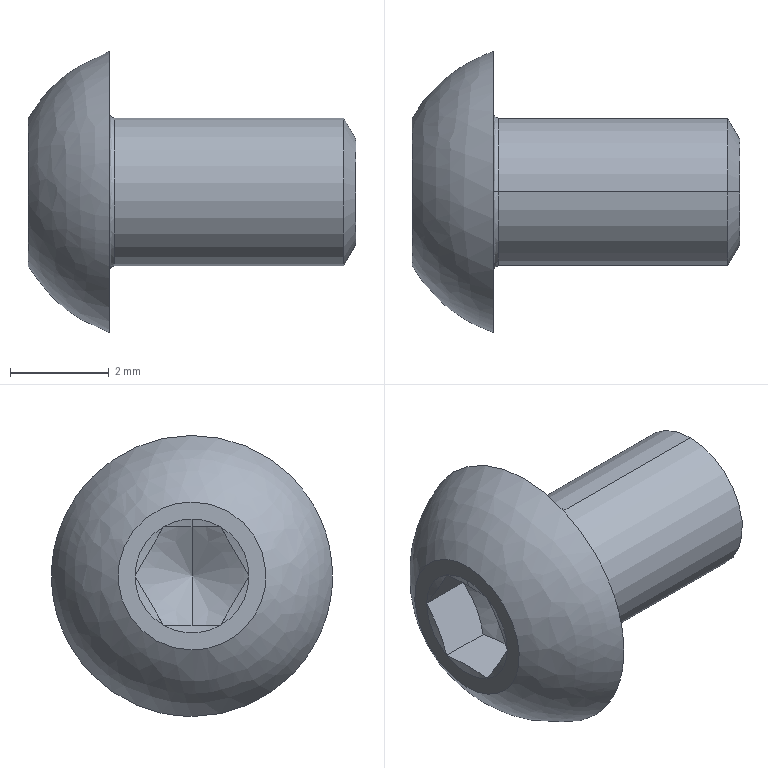Part | SolidWorks | features BaseBody 1 | 1 solid | 25 faces | box 6.65 x 5.7 x 5.7 mm | volume 59.694 mm3 | cone 11 | plane 9 | spline 3 | cylinder 2 | commonest cylinder face diameters 3 x2
STEP:
#1=CARTESIAN_POINT('',(-4.9,0.,-1.5));
#2=VERTEX_POINT('',#1);
#3=CARTESIAN_POINT('',(-4.9,0.,1.5));
#4=VERTEX_POINT('',#3);
#5=CARTESIAN_POINT('',(-4.9,0.,0.));
#6=DIRECTION('',(1.,0.,0.));
#7=DIRECTION('',(0.,0.,1.));
#8=AXIS2_PLACEMENT_3D('',#5,#6,#7);
#9=CIRCLE('',#8,1.5);
#10=EDGE_CURVE('',#2,#4,#9,.T.);
#11=ORIENTED_EDGE('',*,*,#10,.F.);
#12=CARTESIAN_POINT('',(-5.,0.,-1.6));
#13=VERTEX_POINT('',#12);
#14=CARTESIAN_POINT('',(-4.9,0.,-1.6));
#15=DIRECTION('',(0.,-1.,0.));
#16=DIRECTION('',(0.,0.,-1.));
#17=AXIS2_PLACEMENT_3D('',#14,#15,#16);
#18=CIRCLE('',#17,0.1);
#19=EDGE_CURVE('',#2,#13,#18,.T.);
#20=ORIENTED_EDGE('',*,*,#19,.T.);
#21=CARTESIAN_POINT('',(-5.,0.,1.6));
#22=VERTEX_POINT('',#21);
#23=CARTESIAN_POINT('',(-5.,0.,1.6));
#24=CARTESIAN_POINT('',(-5.,0.1018,1.6));
#25=CARTESIAN_POINT('',(-5.,0.2518,1.586));
#26=CARTESIAN_POINT('',(-5.,0.422,1.545));
#27=CARTESIAN_POINT('',(-5.,0.4939,1.522));
#28=CARTESIAN_POINT('',(-5.,0.5416,1.506));
#29=CARTESIAN_POINT('',(-5.,0.5632,1.498));
#30=CARTESIAN_POINT('',(-5.,0.7947,1.406));
#31=CARTESIAN_POINT('',(-5.,0.975,1.288));
#32=CARTESIAN_POINT('',(-5.,1.21,1.053));
#33=CARTESIAN_POINT('',(-5.,1.313,0.9266));
#34=CARTESIAN_POINT('',(-5.,1.408,0.7631));
#35=CARTESIAN_POINT('',(-5.,1.444,0.6896));
#36=CARTESIAN_POINT('',(-5.,1.467,0.6398));
#37=CARTESIAN_POINT('',(-5.,1.478,0.6126));
#38=CARTESIAN_POINT('',(-5.,1.563,0.3994));
#39=CARTESIAN_POINT('',(-5.,1.6,0.2038));
#40=CARTESIAN_POINT('',(-5.,1.6,-0.1019));
#41=CARTESIAN_POINT('',(-5.,1.586,-0.252));
#42=CARTESIAN_POINT('',(-5.,1.545,-0.4221));
#43=CARTESIAN_POINT('',(-5.,1.518,-0.5059));
#44=CARTESIAN_POINT('',(-5.,1.506,-0.5416));
#45=CARTESIAN_POINT('',(-5.,1.497,-0.5653));
#46=CARTESIAN_POINT('',(-5.,1.493,-0.5761));
#47=CARTESIAN_POINT('',(-5.,1.406,-0.7947));
#48=CARTESIAN_POINT('',(-5.,1.288,-0.975));
#49=CARTESIAN_POINT('',(-5.,1.053,-1.21));
#50=CARTESIAN_POINT('',(-5.,0.9266,-1.313));
#51=CARTESIAN_POINT('',(-5.,0.7631,-1.408));
#52=CARTESIAN_POINT('',(-5.,0.6896,-1.444));
#53=CARTESIAN_POINT('',(-5.,0.6398,-1.467));
#54=CARTESIAN_POINT('',(-5.,0.6126,-1.478));
#55=CARTESIAN_POINT('',(-5.,0.3994,-1.563));
#56=CARTESIAN_POINT('',(-5.,0.2038,-1.6));
#57=CARTESIAN_POINT('',(-5.,0.,-1.6));
#58=B_SPLINE_CURVE_WITH_KNOTS('',3,(#23,#24,#25,#26,#27,#28,#29,#30,#31,#32,#33,#34,#35,#36,#37,#38,#39,#40,#41,#42,#43,#44,#45,#46,#47,#48,#49,#50,#51,#52,#53,#54,#55,#56,#57),.UNSPECIFIED.,.F.,.F.,(4,1,1,2,2,2,1,1,2,2,2,1,1,1,2,2,2,1,1,2,2,4),(0.,0.03125,0.04688,0.05469,0.0625,0.125,0.1563,0.1719,0.1797,0.1875,0.25,0.2812,0.2969,0.3047,0.3086,0.3125,0.375,0.4062,0.4219,0.4297,0.4375,0.5),.UNSPECIFIED.);
#59=EDGE_CURVE('',#22,#13,#58,.T.);
#60=ORIENTED_EDGE('',*,*,#59,.F.);
#61=CARTESIAN_POINT('',(-4.9,0.,1.6));
#62=DIRECTION('',(0.,1.,0.));
#63=DIRECTION('',(0.,0.,1.));
#64=AXIS2_PLACEMENT_3D('',#61,#62,#63);
#65=CIRCLE('',#64,0.1);
#66=EDGE_CURVE('',#4,#22,#65,.T.);
#67=ORIENTED_EDGE('',*,*,#66,.F.);
#68=EDGE_LOOP('',(#11,#20,#60,#67));
#69=FACE_OUTER_BOUND('',#68,.T.);
#70=CARTESIAN_POINT('',(-4.9,0.,1.5));
#71=CARTESIAN_POINT('',(-4.9,3.,1.5));
#72=CARTESIAN_POINT('',(-4.9,3.,-1.5));
#73=CARTESIAN_POINT('',(-4.9,0.,-1.5));
#74=CARTESIAN_POINT('',(-4.959,0.,1.5));
#75=CARTESIAN_POINT('',(-4.959,3.,1.5));
#76=CARTESIAN_POINT('',(-4.959,3.,-1.5));
#77=CARTESIAN_POINT('',(-4.959,0.,-1.5));
#78=CARTESIAN_POINT('',(-5.,0.,1.541));
#79=CARTESIAN_POINT('',(-5.,3.083,1.541));
#80=CARTESIAN_POINT('',(-5.,3.083,-1.541));
#81=CARTESIAN_POINT('',(-5.,0.,-1.541));
#82=CARTESIAN_POINT('',(-5.,0.,1.6));
#83=CARTESIAN_POINT('',(-5.,3.2,1.6));
#84=CARTESIAN_POINT('',(-5.,3.2,-1.6));
#85=CARTESIAN_POINT('',(-5.,0.,-1.6));
#86=(BOUNDED_SURFACE()B_SPLINE_SURFACE(3,3,((#70,#71,#72,#73),(#74,#75,#76,#77),(#78,#79,#80,#81),(#82,#83,#84,#85)),.UNSPECIFIED.,.F.,.F.,.F.)B_SPLINE_SURFACE_WITH_KNOTS((4,4),(4,4),(0.,1.),(0.,1.),.UNSPECIFIED.)GEOMETRIC_REPRESENTATION_ITEM()RATIONAL_B_SPLINE_SURFACE(((1.,0.3333,0.3333,1.),(0.8047,0.2682,0.2682,0.8047),(0.8047,0.2682,0.2682,0.8047),(1.,0.3333,0.3333,1.)))REPRESENTATION_ITEM('')SURFACE());
#87=ADVANCED_FACE('',(#69),#86,.F.);
#88=CARTESIAN_POINT('',(-0.25,0.,1.5));
#89=VERTEX_POINT('',#88);
#90=CARTESIAN_POINT('',(-0.25,0.,-1.5));
#91=VERTEX_POINT('',#90);
#92=CARTESIAN_POINT('',(-0.25,0.,0.));
#93=DIRECTION('',(-1.,0.,0.));
#94=DIRECTION('',(0.,0.,1.));
#95=AXIS2_PLACEMENT_3D('',#92,#93,#94);
#96=CIRCLE('',#95,1.5);
#97=EDGE_CURVE('',#89,#91,#96,.T.);
#98=ORIENTED_EDGE('',*,*,#97,.T.);
#99=CARTESIAN_POINT('',(-6.65,0.,-1.5));
#100=DIRECTION('',(-1.,0.,0.));
#101=VECTOR('',#100,1000.);
#102=LINE('',#99,#101);
#103=EDGE_CURVE('',#91,#2,#102,.T.);
#104=ORIENTED_EDGE('',*,*,#103,.T.);
#105=ORIENTED_EDGE('',*,*,#10,.T.);
#106=CARTESIAN_POINT('',(-6.65,0.,1.5));
#107=DIRECTION('',(-1.,0.,0.));
#108=VECTOR('',#107,1000.);
#109=LINE('',#106,#108);
#110=EDGE_CURVE('',#89,#4,#109,.T.);
#111=ORIENTED_EDGE('',*,*,#110,.F.);
#112=EDGE_LOOP('',(#98,#104,#105,#111));
#113=FACE_OUTER_BOUND('',#112,.T.);
#114=CARTESIAN_POINT('',(-6.65,0.,0.));
#115=DIRECTION('',(-1.,0.,0.));
#116=DIRECTION('',(0.,0.,1.));
#117=AXIS2_PLACEMENT_3D('',#114,#115,#116);
#118=CYLINDRICAL_SURFACE('',#117,1.5);
#119=ADVANCED_FACE('',(#113),#118,.T.);
#120=CARTESIAN_POINT('',(0.,0.,1.067));
#121=VERTEX_POINT('',#120);
#122=CARTESIAN_POINT('',(0.,0.,-1.067));
#123=VERTEX_POINT('',#122);
#124=CARTESIAN_POINT('',(0.,0.,0.));
#125=DIRECTION('',(-1.,0.,0.));
#126=DIRECTION('',(0.,0.,1.));
#127=AXIS2_PLACEMENT_3D('',#124,#125,#126);
#128=CIRCLE('',#127,1.067);
#129=EDGE_CURVE('',#121,#123,#128,.T.);
#130=ORIENTED_EDGE('',*,*,#129,.T.);
#131=CARTESIAN_POINT('',(-0.25,0.,-1.5));
#132=DIRECTION('',(-0.5,0.,-0.866));
#133=VECTOR('',#132,1000.);
#134=LINE('',#131,#133);
#135=EDGE_CURVE('',#123,#91,#134,.T.);
#136=ORIENTED_EDGE('',*,*,#135,.T.);
#137=ORIENTED_EDGE('',*,*,#97,.F.);
#138=CARTESIAN_POINT('',(-0.25,0.,1.5));
#139=DIRECTION('',(-0.5,0.,0.866));
#140=VECTOR('',#139,1000.);
#141=LINE('',#138,#140);
#142=EDGE_CURVE('',#121,#89,#141,.T.);
#143=ORIENTED_EDGE('',*,*,#142,.F.);
#144=EDGE_LOOP('',(#130,#136,#137,#143));
#145=FACE_OUTER_BOUND('',#144,.T.);
#146=CARTESIAN_POINT('',(-0.25,0.,0.));
#147=DIRECTION('',(-1.,0.,0.));
#148=DIRECTION('',(0.,0.,1.));
#149=AXIS2_PLACEMENT_3D('',#146,#147,#148);
#150=CONICAL_SURFACE('',#149,1.5,1.047);
#151=ADVANCED_FACE('',(#145),#150,.T.);
#152=CARTESIAN_POINT('',(-6.61,0.,1.));
#153=VERTEX_POINT('',#152);
#154=CARTESIAN_POINT('',(-6.65,0.5774,1.));
#155=VERTEX_POINT('',#154);
#156=CARTESIAN_POINT('',(-6.61,0.,1.));
#157=CARTESIAN_POINT('',(-6.61,0.1925,1.));
#158=CARTESIAN_POINT('',(-6.625,0.3849,1.));
#159=CARTESIAN_POINT('',(-6.65,0.5774,1.));
#160=B_SPLINE_CURVE_WITH_KNOTS('',3,(#156,#157,#158,#159),.UNSPECIFIED.,.F.,.F.,(4,4),(0.0005774,0.001155),.UNSPECIFIED.);
#161=EDGE_CURVE('',#153,#155,#160,.T.);
#162=ORIENTED_EDGE('',*,*,#161,.F.);
#163=CARTESIAN_POINT('',(-6.65,0.,1.155));
#164=VERTEX_POINT('',#163);
#165=CARTESIAN_POINT('',(-6.65,0.,1.155));
#166=DIRECTION('',(-0.2515,0.,0.9679));
#167=VECTOR('',#166,1000.);
#168=LINE('',#165,#167);
#169=EDGE_CURVE('',#153,#164,#168,.T.);
#170=ORIENTED_EDGE('',*,*,#169,.T.);
#171=CARTESIAN_POINT('',(-6.65,0.,0.));
#172=DIRECTION('',(-1.,0.,0.));
#173=DIRECTION('',(0.,0.,1.));
#174=AXIS2_PLACEMENT_3D('',#171,#172,#173);
#175=CIRCLE('',#174,1.155);
#176=EDGE_CURVE('',#164,#155,#175,.T.);
#177=ORIENTED_EDGE('',*,*,#176,.T.);
#178=EDGE_LOOP('',(#162,#170,#177));
#179=FACE_OUTER_BOUND('',#178,.T.);
#180=CARTESIAN_POINT('',(-6.65,0.,0.));
#181=DIRECTION('',(-1.,0.,0.));
#182=DIRECTION('',(0.,0.,1.));
#183=AXIS2_PLACEMENT_3D('',#180,#181,#182);
#184=CONICAL_SURFACE('',#183,1.155,1.317);
#185=ADVANCED_FACE('',(#179),#184,.F.);
#186=CARTESIAN_POINT('',(-5.,0.,0.));
#187=VERTEX_POINT('',#186);
#188=CARTESIAN_POINT('',(-5.528,0.,1.));
#189=VERTEX_POINT('',#188);
#190=CARTESIAN_POINT('',(-5.614,0.,1.162));
#191=DIRECTION('',(-0.4671,0.,0.8842));
#192=VECTOR('',#191,1000.);
#193=LINE('',#190,#192);
#194=EDGE_CURVE('',#187,#189,#193,.T.);
#195=ORIENTED_EDGE('',*,*,#194,.F.);
#196=CARTESIAN_POINT('',(-5.528,0.,-1.));
#197=VERTEX_POINT('',#196);
#198=CARTESIAN_POINT('',(-5.614,0.,-1.162));
#199=DIRECTION('',(-0.4671,0.,-0.8842));
#200=VECTOR('',#199,1000.);
#201=LINE('',#198,#200);
#202=EDGE_CURVE('',#187,#197,#201,.T.);
#203=ORIENTED_EDGE('',*,*,#202,.T.);
#204=CARTESIAN_POINT('',(-5.61,-0.5774,-1.));
#205=VERTEX_POINT('',#204);
#206=CARTESIAN_POINT('',(-5.528,0.,-1.));
#207=CARTESIAN_POINT('',(-5.528,-0.1955,-1.));
#208=CARTESIAN_POINT('',(-5.56,-0.3883,-1.));
#209=CARTESIAN_POINT('',(-5.61,-0.5774,-1.));
#210=B_SPLINE_CURVE_WITH_KNOTS('',3,(#206,#207,#208,#209),.UNSPECIFIED.,.F.,.F.,(4,4),(0.0005831,0.001165),.UNSPECIFIED.);
#211=EDGE_CURVE('',#197,#205,#210,.T.);
#212=ORIENTED_EDGE('',*,*,#211,.T.);
#213=CARTESIAN_POINT('',(-5.61,-1.155,0.));
#214=VERTEX_POINT('',#213);
#215=CARTESIAN_POINT('',(-5.61,-0.5774,-1.));
#216=CARTESIAN_POINT('',(-5.56,-0.6719,-0.8362));
#217=CARTESIAN_POINT('',(-5.528,-0.7677,-0.6702));
#218=CARTESIAN_POINT('',(-5.528,-0.9635,-0.3311));
#219=CARTESIAN_POINT('',(-5.56,-1.06,-0.164));
#220=CARTESIAN_POINT('',(-5.61,-1.155,0.));
#221=B_SPLINE_CURVE_WITH_KNOTS('',3,(#215,#216,#217,#218,#219,#220),.UNSPECIFIED.,.F.,.F.,(4,2,4),(0.,0.0005823,0.001165),.UNSPECIFIED.);
#222=EDGE_CURVE('',#205,#214,#221,.T.);
#223=ORIENTED_EDGE('',*,*,#222,.T.);
#224=CARTESIAN_POINT('',(-5.61,-0.5774,1.));
#225=VERTEX_POINT('',#224);
#226=CARTESIAN_POINT('',(-5.61,-1.155,0.));
#227=CARTESIAN_POINT('',(-5.56,-1.06,0.1638));
#228=CARTESIAN_POINT('',(-5.528,-0.9643,0.3298));
#229=CARTESIAN_POINT('',(-5.528,-0.7685,0.6689));
#230=CARTESIAN_POINT('',(-5.56,-0.672,0.836));
#231=CARTESIAN_POINT('',(-5.61,-0.5774,1.));
#232=B_SPLINE_CURVE_WITH_KNOTS('',3,(#226,#227,#228,#229,#230,#231),.UNSPECIFIED.,.F.,.F.,(4,2,4),(0.,0.0005823,0.001165),.UNSPECIFIED.);
#233=EDGE_CURVE('',#214,#225,#232,.T.);
#234=ORIENTED_EDGE('',*,*,#233,.T.);
#235=CARTESIAN_POINT('',(-5.61,-0.5774,1.));
#236=CARTESIAN_POINT('',(-5.56,-0.3879,1.));
#237=CARTESIAN_POINT('',(-5.528,-0.1961,1.));
#238=CARTESIAN_POINT('',(-5.528,0.,1.));
#239=B_SPLINE_CURVE_WITH_KNOTS('',3,(#235,#236,#237,#238),.UNSPECIFIED.,.F.,.F.,(4,4),(0.,0.0005831),.UNSPECIFIED.);
#240=EDGE_CURVE('',#225,#189,#239,.T.);
#241=ORIENTED_EDGE('',*,*,#240,.T.);
#242=EDGE_LOOP('',(#195,#203,#212,#223,#234,#241));
#243=FACE_OUTER_BOUND('',#242,.T.);
#244=CARTESIAN_POINT('',(-5.614,0.,0.));
#245=DIRECTION('',(-1.,0.,0.));
#246=DIRECTION('',(0.,0.,1.));
#247=AXIS2_PLACEMENT_3D('',#244,#245,#246);
#248=CONICAL_SURFACE('',#247,1.162,1.085);
#249=ADVANCED_FACE('',(#243),#248,.F.);
#250=ORIENTED_EDGE('',*,*,#103,.F.);
#251=CARTESIAN_POINT('',(-0.25,0.,0.));
#252=DIRECTION('',(-1.,0.,0.));
#253=DIRECTION('',(0.,0.,1.));
#254=AXIS2_PLACEMENT_3D('',#251,#252,#253);
#255=CIRCLE('',#254,1.5);
#256=EDGE_CURVE('',#91,#89,#255,.T.);
#257=ORIENTED_EDGE('',*,*,#256,.T.);
#258=ORIENTED_EDGE('',*,*,#110,.T.);
#259=CARTESIAN_POINT('',(-4.9,0.,0.));
#260=DIRECTION('',(1.,0.,0.));
#261=DIRECTION('',(0.,0.,1.));
#262=AXIS2_PLACEMENT_3D('',#259,#260,#261);
#263=CIRCLE('',#262,1.5);
#264=EDGE_CURVE('',#4,#2,#263,.T.);
#265=ORIENTED_EDGE('',*,*,#264,.T.);
#266=EDGE_LOOP('',(#250,#257,#258,#265));
#267=FACE_OUTER_BOUND('',#266,.T.);
#268=CARTESIAN_POINT('',(-6.65,0.,0.));
#269=DIRECTION('',(-1.,0.,0.));
#270=DIRECTION('',(0.,0.,1.));
#271=AXIS2_PLACEMENT_3D('',#268,#269,#270);
#272=CYLINDRICAL_SURFACE('',#271,1.5);
#273=ADVANCED_FACE('',(#267),#272,.T.);
#274=ORIENTED_EDGE('',*,*,#135,.F.);
#275=CARTESIAN_POINT('',(0.,0.,0.));
#276=DIRECTION('',(-1.,0.,0.));
#277=DIRECTION('',(0.,0.,1.));
#278=AXIS2_PLACEMENT_3D('',#275,#276,#277);
#279=CIRCLE('',#278,1.067);
#280=EDGE_CURVE('',#123,#121,#279,.T.);
#281=ORIENTED_EDGE('',*,*,#280,.T.);
#282=ORIENTED_EDGE('',*,*,#142,.T.);
#283=ORIENTED_EDGE('',*,*,#256,.F.);
#284=EDGE_LOOP('',(#274,#281,#282,#283));
#285=FACE_OUTER_BOUND('',#284,.T.);
#286=CARTESIAN_POINT('',(-0.25,0.,0.));
#287=DIRECTION('',(-1.,0.,0.));
#288=DIRECTION('',(0.,0.,1.));
#289=AXIS2_PLACEMENT_3D('',#286,#287,#288);
#290=CONICAL_SURFACE('',#289,1.5,1.047);
#291=ADVANCED_FACE('',(#285),#290,.T.);
#292=ORIENTED_EDGE('',*,*,#19,.F.);
#293=ORIENTED_EDGE('',*,*,#264,.F.);
#294=ORIENTED_EDGE('',*,*,#66,.T.);
#295=CARTESIAN_POINT('',(-5.,0.,-1.6));
#296=CARTESIAN_POINT('',(-5.,-0.1019,-1.6));
#297=CARTESIAN_POINT('',(-5.,-0.252,-1.586));
#298=CARTESIAN_POINT('',(-5.,-0.4221,-1.545));
#299=CARTESIAN_POINT('',(-5.,-0.5059,-1.518));
#300=CARTESIAN_POINT('',(-5.,-0.5416,-1.506));
#301=CARTESIAN_POINT('',(-5.,-0.5653,-1.497));
#302=CARTESIAN_POINT('',(-5.,-0.5761,-1.493));
#303=CARTESIAN_POINT('',(-5.,-0.7947,-1.406));
#304=CARTESIAN_POINT('',(-5.,-0.975,-1.288));
#305=CARTESIAN_POINT('',(-5.,-1.21,-1.053));
#306=CARTESIAN_POINT('',(-5.,-1.313,-0.9266));
#307=CARTESIAN_POINT('',(-5.,-1.408,-0.7631));
#308=CARTESIAN_POINT('',(-5.,-1.444,-0.6896));
#309=CARTESIAN_POINT('',(-5.,-1.467,-0.6398));
#310=CARTESIAN_POINT('',(-5.,-1.478,-0.6126));
#311=CARTESIAN_POINT('',(-5.,-1.563,-0.3994));
#312=CARTESIAN_POINT('',(-5.,-1.6,-0.2038));
#313=CARTESIAN_POINT('',(-5.,-1.6,0.1019));
#314=CARTESIAN_POINT('',(-5.,-1.586,0.252));
#315=CARTESIAN_POINT('',(-5.,-1.545,0.4221));
#316=CARTESIAN_POINT('',(-5.,-1.518,0.5059));
#317=CARTESIAN_POINT('',(-5.,-1.506,0.5416));
#318=CARTESIAN_POINT('',(-5.,-1.497,0.5653));
#319=CARTESIAN_POINT('',(-5.,-1.493,0.5761));
#320=CARTESIAN_POINT('',(-5.,-1.406,0.7947));
#321=CARTESIAN_POINT('',(-5.,-1.288,0.975));
#322=CARTESIAN_POINT('',(-5.,-1.053,1.21));
#323=CARTESIAN_POINT('',(-5.,-0.9266,1.313));
#324=CARTESIAN_POINT('',(-5.,-0.7631,1.408));
#325=CARTESIAN_POINT('',(-5.,-0.6896,1.444));
#326=CARTESIAN_POINT('',(-5.,-0.6398,1.467));
#327=CARTESIAN_POINT('',(-5.,-0.6126,1.478));
#328=CARTESIAN_POINT('',(-5.,-0.3996,1.563));
#329=CARTESIAN_POINT('',(-5.,-0.2033,1.6));
#330=CARTESIAN_POINT('',(-5.,0.,1.6));
#331=B_SPLINE_CURVE_WITH_KNOTS('',3,(#295,#296,#297,#298,#299,#300,#301,#302,#303,#304,#305,#306,#307,#308,#309,#310,#311,#312,#313,#314,#315,#316,#317,#318,#319,#320,#321,#322,#323,#324,#325,#326,#327,#328,#329,#330),.UNSPECIFIED.,.F.,.F.,(4,1,1,1,2,2,2,1,1,2,2,2,1,1,1,2,2,2,1,1,2,2,4),(0.5,0.5312,0.5469,0.5547,0.5586,0.5625,0.625,0.6562,0.6719,0.6797,0.6875,0.75,0.7812,0.7969,0.8047,0.8086,0.8125,0.875,0.9062,0.9219,0.9297,0.9375,1.),.UNSPECIFIED.);
#332=EDGE_CURVE('',#13,#22,#331,.T.);
#333=ORIENTED_EDGE('',*,*,#332,.F.);
#334=EDGE_LOOP('',(#292,#293,#294,#333));
#335=FACE_OUTER_BOUND('',#334,.T.);
#336=CARTESIAN_POINT('',(-4.9,0.,-1.5));
#337=CARTESIAN_POINT('',(-4.9,-3.,-1.5));
#338=CARTESIAN_POINT('',(-4.9,-3.,1.5));
#339=CARTESIAN_POINT('',(-4.9,0.,1.5));
#340=CARTESIAN_POINT('',(-4.959,0.,-1.5));
#341=CARTESIAN_POINT('',(-4.959,-3.,-1.5));
#342=CARTESIAN_POINT('',(-4.959,-3.,1.5));
#343=CARTESIAN_POINT('',(-4.959,0.,1.5));
#344=CARTESIAN_POINT('',(-5.,0.,-1.541));
#345=CARTESIAN_POINT('',(-5.,-3.083,-1.541));
#346=CARTESIAN_POINT('',(-5.,-3.083,1.541));
#347=CARTESIAN_POINT('',(-5.,0.,1.541));
#348=CARTESIAN_POINT('',(-5.,0.,-1.6));
#349=CARTESIAN_POINT('',(-5.,-3.2,-1.6));
#350=CARTESIAN_POINT('',(-5.,-3.2,1.6));
#351=CARTESIAN_POINT('',(-5.,0.,1.6));
#352=(BOUNDED_SURFACE()B_SPLINE_SURFACE(3,3,((#336,#337,#338,#339),(#340,#341,#342,#343),(#344,#345,#346,#347),(#348,#349,#350,#351)),.UNSPECIFIED.,.F.,.F.,.F.)B_SPLINE_SURFACE_WITH_KNOTS((4,4),(4,4),(0.,1.),(0.,1.),.UNSPECIFIED.)GEOMETRIC_REPRESENTATION_ITEM()RATIONAL_B_SPLINE_SURFACE(((1.,0.3333,0.3333,1.),(0.8047,0.2682,0.2682,0.8047),(0.8047,0.2682,0.2682,0.8047),(1.,0.3333,0.3333,1.)))REPRESENTATION_ITEM('')SURFACE());
#353=ADVANCED_FACE('',(#335),#352,.F.);
#354=ORIENTED_EDGE('',*,*,#129,.F.);
#355=ORIENTED_EDGE('',*,*,#280,.F.);
#356=EDGE_LOOP('',(#354,#355));
#357=FACE_OUTER_BOUND('',#356,.T.);
#358=CARTESIAN_POINT('',(0.,1.5,0.));
#359=DIRECTION('',(-1.,0.,0.));
#360=DIRECTION('',(0.,0.,1.));
#361=AXIS2_PLACEMENT_3D('',#358,#359,#360);
#362=PLANE('',#361);
#363=ADVANCED_FACE('',(#357),#362,.F.);
#364=ORIENTED_EDGE('',*,*,#59,.T.);
#365=ORIENTED_EDGE('',*,*,#332,.T.);
#366=EDGE_LOOP('',(#364,#365));
#367=FACE_BOUND('',#366,.T.);
#368=CARTESIAN_POINT('',(-5.,0.,-2.85));
#369=VERTEX_POINT('',#368);
#370=CARTESIAN_POINT('',(-5.,0.001007,2.85));
#371=VERTEX_POINT('',#370);
#372=CARTESIAN_POINT('',(-5.,0.,-2.85));
#373=CARTESIAN_POINT('',(-5.,-0.3766,-2.85));
#374=CARTESIAN_POINT('',(-5.,-0.7506,-2.774));
#375=CARTESIAN_POINT('',(-5.,-1.265,-2.561));
#376=CARTESIAN_POINT('',(-5.,-1.431,-2.472));
#377=CARTESIAN_POINT('',(-5.,-1.742,-2.263));
#378=CARTESIAN_POINT('',(-5.,-1.885,-2.145));
#379=CARTESIAN_POINT('',(-5.,-2.148,-1.882));
#380=CARTESIAN_POINT('',(-5.,-2.269,-1.735));
#381=CARTESIAN_POINT('',(-5.,-2.475,-1.425));
#382=CARTESIAN_POINT('',(-5.,-2.562,-1.262));
#383=CARTESIAN_POINT('',(-5.,-2.705,-0.9158));
#384=CARTESIAN_POINT('',(-5.,-2.76,-0.7352));
#385=CARTESIAN_POINT('',(-5.,-2.832,-0.371));
#386=CARTESIAN_POINT('',(-5.,-2.85,-0.185));
#387=CARTESIAN_POINT('',(-5.,-2.85,0.1908));
#388=CARTESIAN_POINT('',(-5.,-2.831,0.3758));
#389=CARTESIAN_POINT('',(-5.,-2.758,0.7401));
#390=CARTESIAN_POINT('',(-5.,-2.703,0.9214));
#391=CARTESIAN_POINT('',(-5.,-2.56,1.266));
#392=CARTESIAN_POINT('',(-5.,-2.473,1.43));
#393=CARTESIAN_POINT('',(-5.,-2.265,1.74));
#394=CARTESIAN_POINT('',(-5.,-2.145,1.886));
#395=CARTESIAN_POINT('',(-5.,-1.882,2.148));
#396=CARTESIAN_POINT('',(-5.,-1.738,2.266));
#397=CARTESIAN_POINT('',(-5.,-1.426,2.475));
#398=CARTESIAN_POINT('',(-5.,-1.26,2.563));
#399=CARTESIAN_POINT('',(-5.,-0.9174,2.705));
#400=CARTESIAN_POINT('',(-5.,-0.7372,2.759));
#401=CARTESIAN_POINT('',(-5.,-0.3698,2.832));
#402=CARTESIAN_POINT('',(-5.,-0.185,2.85));
#403=CARTESIAN_POINT('',(-5.,0.001007,2.85));
#404=B_SPLINE_CURVE_WITH_KNOTS('',3,(#372,#373,#374,#375,#376,#377,#378,#379,#380,#381,#382,#383,#384,#385,#386,#387,#388,#389,#390,#391,#392,#393,#394,#395,#396,#397,#398,#399,#400,#401,#402,#403),.UNSPECIFIED.,.F.,.F.,(4,2,2,2,2,2,2,2,2,2,2,2,2,2,2,4),(0.,0.001123,0.001685,0.002247,0.002809,0.00337,0.003932,0.004494,0.005056,0.005617,0.006179,0.006741,0.007302,0.007864,0.008426,0.008988),.UNSPECIFIED.);
#405=EDGE_CURVE('',#369,#371,#404,.T.);
#406=ORIENTED_EDGE('',*,*,#405,.F.);
#407=CARTESIAN_POINT('',(-5.,0.001007,2.85));
#408=CARTESIAN_POINT('',(-5.,0.187,2.85));
#409=CARTESIAN_POINT('',(-5.,0.3759,2.831));
#410=CARTESIAN_POINT('',(-5.,0.741,2.758));
#411=CARTESIAN_POINT('',(-5.,0.9186,2.704));
#412=CARTESIAN_POINT('',(-5.,1.264,2.561));
#413=CARTESIAN_POINT('',(-5.,1.43,2.472));
#414=CARTESIAN_POINT('',(-5.,1.739,2.266));
#415=CARTESIAN_POINT('',(-5.,1.883,2.147));
#416=CARTESIAN_POINT('',(-5.,2.149,1.881));
#417=CARTESIAN_POINT('',(-5.,2.267,1.737));
#418=CARTESIAN_POINT('',(-5.,2.473,1.428));
#419=CARTESIAN_POINT('',(-5.,2.562,1.261));
#420=CARTESIAN_POINT('',(-5.,2.705,0.9163));
#421=CARTESIAN_POINT('',(-5.,2.759,0.7387));
#422=CARTESIAN_POINT('',(-5.,2.832,0.3731));
#423=CARTESIAN_POINT('',(-5.,2.85,0.1844));
#424=CARTESIAN_POINT('',(-5.,2.85,-0.1874));
#425=CARTESIAN_POINT('',(-5.,2.832,-0.3723));
#426=CARTESIAN_POINT('',(-5.,2.759,-0.7402));
#427=CARTESIAN_POINT('',(-5.,2.704,-0.9197));
#428=CARTESIAN_POINT('',(-5.,2.562,-1.263));
#429=CARTESIAN_POINT('',(-5.,2.473,-1.429));
#430=CARTESIAN_POINT('',(-5.,2.265,-1.74));
#431=CARTESIAN_POINT('',(-5.,2.147,-1.884));
#432=CARTESIAN_POINT('',(-5.,1.884,-2.147));
#433=CARTESIAN_POINT('',(-5.,1.737,-2.267));
#434=CARTESIAN_POINT('',(-5.,1.427,-2.474));
#435=CARTESIAN_POINT('',(-5.,1.264,-2.561));
#436=CARTESIAN_POINT('',(-5.,0.9187,-2.704));
#437=CARTESIAN_POINT('',(-5.,0.7377,-2.759));
#438=CARTESIAN_POINT('',(-5.,0.3734,-2.832));
#439=CARTESIAN_POINT('',(-5.,0.1883,-2.85));
#440=CARTESIAN_POINT('',(-5.,0.,-2.85));
#441=B_SPLINE_CURVE_WITH_KNOTS('',3,(#407,#408,#409,#410,#411,#412,#413,#414,#415,#416,#417,#418,#419,#420,#421,#422,#423,#424,#425,#426,#427,#428,#429,#430,#431,#432,#433,#434,#435,#436,#437,#438,#439,#440),.UNSPECIFIED.,.F.,.F.,(4,2,2,2,2,2,2,2,2,2,2,2,2,2,2,2,4),(0.008988,0.009549,0.01011,0.01067,0.01123,0.0118,0.01236,0.01292,0.01348,0.01404,0.0146,0.01517,0.01573,0.01629,0.01685,0.01741,0.01798),.UNSPECIFIED.);
#442=EDGE_CURVE('',#371,#369,#441,.T.);
#443=ORIENTED_EDGE('',*,*,#442,.F.);
#444=EDGE_LOOP('',(#406,#443));
#445=FACE_OUTER_BOUND('',#444,.T.);
#446=CARTESIAN_POINT('',(-5.,1.6,0.));
#447=DIRECTION('',(-1.,0.,0.));
#448=DIRECTION('',(0.,0.,1.));
#449=AXIS2_PLACEMENT_3D('',#446,#447,#448);
#450=PLANE('',#449);
#451=ADVANCED_FACE('',(#367,#445),#450,.F.);
#452=ORIENTED_EDGE('',*,*,#405,.T.);
#453=ORIENTED_EDGE('',*,*,#442,.T.);
#454=EDGE_LOOP('',(#452,#453));
#455=FACE_OUTER_BOUND('',#454,.T.);
#456=CARTESIAN_POINT('',(-6.65,0.,-1.5));
#457=VERTEX_POINT('',#456);
#458=CARTESIAN_POINT('',(-6.65,-0.0005302,1.5));
#459=VERTEX_POINT('',#458);
#460=CARTESIAN_POINT('',(-6.65,0.,-1.5));
#461=CARTESIAN_POINT('',(-6.65,0.1982,-1.5));
#462=CARTESIAN_POINT('',(-6.65,0.3951,-1.46));
#463=CARTESIAN_POINT('',(-6.65,0.756,-1.31));
#464=CARTESIAN_POINT('',(-6.65,0.9231,-1.198));
#465=CARTESIAN_POINT('',(-6.65,1.131,-0.9905));
#466=CARTESIAN_POINT('',(-6.65,1.194,-0.9132));
#467=CARTESIAN_POINT('',(-6.65,1.303,-0.7502));
#468=CARTESIAN_POINT('',(-6.65,1.349,-0.664));
#469=CARTESIAN_POINT('',(-6.65,1.461,-0.391));
#470=CARTESIAN_POINT('',(-6.65,1.5,-0.1963));
#471=CARTESIAN_POINT('',(-6.65,1.5,0.1004));
#472=CARTESIAN_POINT('',(-6.65,1.49,0.1978));
#473=CARTESIAN_POINT('',(-6.65,1.452,0.3895));
#474=CARTESIAN_POINT('',(-6.65,1.423,0.4849));
#475=CARTESIAN_POINT('',(-6.65,1.347,0.6663));
#476=CARTESIAN_POINT('',(-6.65,1.301,0.7524));
#477=CARTESIAN_POINT('',(-6.65,1.192,0.9155));
#478=CARTESIAN_POINT('',(-6.65,1.129,0.9926));
#479=CARTESIAN_POINT('',(-6.65,0.9212,1.2));
#480=CARTESIAN_POINT('',(-6.65,0.7537,1.312));
#481=CARTESIAN_POINT('',(-6.65,0.3926,1.461));
#482=CARTESIAN_POINT('',(-6.65,0.1952,1.5));
#483=CARTESIAN_POINT('',(-6.65,-0.0005302,1.5));
#484=B_SPLINE_CURVE_WITH_KNOTS('',3,(#460,#461,#462,#463,#464,#465,#466,#467,#468,#469,#470,#471,#472,#473,#474,#475,#476,#477,#478,#479,#480,#481,#482,#483),.UNSPECIFIED.,.F.,.F.,(4,2,2,2,2,2,2,2,2,2,2,4),(0.,0.0005913,0.001183,0.001478,0.001774,0.002365,0.002661,0.002956,0.003252,0.003548,0.004139,0.00473),.UNSPECIFIED.);
#485=EDGE_CURVE('',#457,#459,#484,.T.);
#486=ORIENTED_EDGE('',*,*,#485,.T.);
#487=CARTESIAN_POINT('',(-6.65,-0.0005302,1.5));
#488=CARTESIAN_POINT('',(-6.65,-0.09842,1.5));
#489=CARTESIAN_POINT('',(-6.65,-0.1978,1.49));
#490=CARTESIAN_POINT('',(-6.65,-0.39,1.452));
#491=CARTESIAN_POINT('',(-6.65,-0.4835,1.423));
#492=CARTESIAN_POINT('',(-6.65,-0.7562,1.31));
#493=CARTESIAN_POINT('',(-6.65,-0.9213,1.2));
#494=CARTESIAN_POINT('',(-6.65,-1.131,0.9901));
#495=CARTESIAN_POINT('',(-6.65,-1.193,0.9143));
#496=CARTESIAN_POINT('',(-6.65,-1.302,0.7517));
#497=CARTESIAN_POINT('',(-6.65,-1.349,0.6639));
#498=CARTESIAN_POINT('',(-6.65,-1.424,0.4823));
#499=CARTESIAN_POINT('',(-6.65,-1.452,0.3888));
#500=CARTESIAN_POINT('',(-6.65,-1.49,0.1964));
#501=CARTESIAN_POINT('',(-6.65,-1.5,0.09703));
#502=CARTESIAN_POINT('',(-6.65,-1.5,-0.1964));
#503=CARTESIAN_POINT('',(-6.65,-1.461,-0.3938));
#504=CARTESIAN_POINT('',(-6.65,-1.311,-0.7548));
#505=CARTESIAN_POINT('',(-6.65,-1.199,-0.9222));
#506=CARTESIAN_POINT('',(-6.65,-0.9916,-1.13));
#507=CARTESIAN_POINT('',(-6.65,-0.9144,-1.193));
#508=CARTESIAN_POINT('',(-6.65,-0.7513,-1.302));
#509=CARTESIAN_POINT('',(-6.65,-0.6652,-1.348));
#510=CARTESIAN_POINT('',(-6.65,-0.4835,-1.423));
#511=CARTESIAN_POINT('',(-6.65,-0.3882,-1.452));
#512=CARTESIAN_POINT('',(-6.65,-0.1965,-1.49));
#513=CARTESIAN_POINT('',(-6.65,-0.0991,-1.5));
#514=CARTESIAN_POINT('',(-6.65,0.,-1.5));
#515=B_SPLINE_CURVE_WITH_KNOTS('',3,(#487,#488,#489,#490,#491,#492,#493,#494,#495,#496,#497,#498,#499,#500,#501,#502,#503,#504,#505,#506,#507,#508,#509,#510,#511,#512,#513,#514),.UNSPECIFIED.,.F.,.F.,(4,2,2,2,2,2,2,2,2,2,2,2,2,4),(0.00473,0.005026,0.005322,0.005913,0.006209,0.006504,0.0068,0.007096,0.007687,0.008278,0.008574,0.008869,0.009165,0.009461),.UNSPECIFIED.);
#516=EDGE_CURVE('',#459,#457,#515,.T.);
#517=ORIENTED_EDGE('',*,*,#516,.T.);
#518=EDGE_LOOP('',(#486,#517));
#519=FACE_BOUND('',#518,.T.);
#520=CARTESIAN_POINT('',(-4.307,2.879,-0.8218));
#521=CARTESIAN_POINT('',(-5.283,2.879,-0.511));
#522=CARTESIAN_POINT('',(-5.282,2.879,0.5134));
#523=CARTESIAN_POINT('',(-4.306,2.879,0.8223));
#524=CARTESIAN_POINT('',(-5.359,1.84,-4.127));
#525=CARTESIAN_POINT('',(-10.262,1.84,-2.567));
#526=CARTESIAN_POINT('',(-10.257,1.84,2.578));
#527=CARTESIAN_POINT('',(-5.351,1.84,4.13));
#528=CARTESIAN_POINT('',(-5.367,-1.781,-4.151));
#529=CARTESIAN_POINT('',(-10.297,-1.781,-2.581));
#530=CARTESIAN_POINT('',(-10.292,-1.781,2.593));
#531=CARTESIAN_POINT('',(-5.359,-1.781,4.153));
#532=CARTESIAN_POINT('',(-4.319,-2.867,-0.8591));
#533=CARTESIAN_POINT('',(-5.339,-2.867,-0.5342));
#534=CARTESIAN_POINT('',(-5.338,-2.867,0.5367));
#535=CARTESIAN_POINT('',(-4.317,-2.867,0.8596));
#536=(BOUNDED_SURFACE()B_SPLINE_SURFACE(3,3,((#520,#521,#522,#523),(#524,#525,#526,#527),(#528,#529,#530,#531),(#532,#533,#534,#535)),.UNSPECIFIED.,.F.,.F.,.F.)B_SPLINE_SURFACE_WITH_KNOTS((4,4),(4,4),(0.,1.),(0.,1.),.UNSPECIFIED.)GEOMETRIC_REPRESENTATION_ITEM()RATIONAL_B_SPLINE_SURFACE(((1.,0.535,0.535,1.),(0.529,0.283,0.283,0.529),(0.529,0.283,0.283,0.529),(1.,0.535,0.535,1.)))REPRESENTATION_ITEM('')SURFACE());
#537=ADVANCED_FACE('',(#455,#519),#536,.T.);
#538=CARTESIAN_POINT('',(-6.65,0.5774,-1.));
#539=VERTEX_POINT('',#538);
#540=CARTESIAN_POINT('',(-6.65,-0.5774,-1.));
#541=VERTEX_POINT('',#540);
#542=CARTESIAN_POINT('',(-6.65,0.,0.));
#543=DIRECTION('',(-1.,0.,0.));
#544=DIRECTION('',(0.,0.,1.));
#545=AXIS2_PLACEMENT_3D('',#542,#543,#544);
#546=CIRCLE('',#545,1.155);
#547=EDGE_CURVE('',#539,#541,#546,.T.);
#548=ORIENTED_EDGE('',*,*,#547,.F.);
#549=CARTESIAN_POINT('',(-6.65,1.155,0.));
#550=VERTEX_POINT('',#549);
#551=CARTESIAN_POINT('',(-6.65,0.,0.));
#552=DIRECTION('',(-1.,0.,0.));
#553=DIRECTION('',(0.,0.,1.));
#554=AXIS2_PLACEMENT_3D('',#551,#552,#553);
#555=CIRCLE('',#554,1.155);
#556=EDGE_CURVE('',#550,#539,#555,.T.);
#557=ORIENTED_EDGE('',*,*,#556,.F.);
#558=CARTESIAN_POINT('',(-6.65,0.,0.));
#559=DIRECTION('',(-1.,0.,0.));
#560=DIRECTION('',(0.,0.,1.));
#561=AXIS2_PLACEMENT_3D('',#558,#559,#560);
#562=CIRCLE('',#561,1.155);
#563=EDGE_CURVE('',#155,#550,#562,.T.);
#564=ORIENTED_EDGE('',*,*,#563,.F.);
#565=ORIENTED_EDGE('',*,*,#176,.F.);
#566=CARTESIAN_POINT('',(-6.65,-0.5774,1.));
#567=VERTEX_POINT('',#566);
#568=CARTESIAN_POINT('',(-6.65,0.,0.));
#569=DIRECTION('',(-1.,0.,0.));
#570=DIRECTION('',(0.,0.,1.));
#571=AXIS2_PLACEMENT_3D('',#568,#569,#570);
#572=CIRCLE('',#571,1.155);
#573=EDGE_CURVE('',#567,#164,#572,.T.);
#574=ORIENTED_EDGE('',*,*,#573,.F.);
#575=CARTESIAN_POINT('',(-6.65,-1.155,0.));
#576=VERTEX_POINT('',#575);
#577=CARTESIAN_POINT('',(-6.65,0.,0.));
#578=DIRECTION('',(-1.,0.,0.));
#579=DIRECTION('',(0.,0.,1.));
#580=AXIS2_PLACEMENT_3D('',#577,#578,#579);
#581=CIRCLE('',#580,1.155);
#582=EDGE_CURVE('',#576,#567,#581,.T.);
#583=ORIENTED_EDGE('',*,*,#582,.F.);
#584=CARTESIAN_POINT('',(-6.65,0.,0.));
#585=DIRECTION('',(-1.,0.,0.));
#586=DIRECTION('',(0.,0.,1.));
#587=AXIS2_PLACEMENT_3D('',#584,#585,#586);
#588=CIRCLE('',#587,1.155);
#589=EDGE_CURVE('',#541,#576,#588,.T.);
#590=ORIENTED_EDGE('',*,*,#589,.F.);
#591=EDGE_LOOP('',(#548,#557,#564,#565,#574,#583,#590));
#592=FACE_BOUND('',#591,.T.);
#593=ORIENTED_EDGE('',*,*,#485,.F.);
#594=ORIENTED_EDGE('',*,*,#516,.F.);
#595=EDGE_LOOP('',(#593,#594));
#596=FACE_OUTER_BOUND('',#595,.T.);
#597=CARTESIAN_POINT('',(-6.65,0.,0.));
#598=DIRECTION('',(1.,0.,0.));
#599=DIRECTION('',(0.,0.,-1.));
#600=AXIS2_PLACEMENT_3D('',#597,#598,#599);
#601=PLANE('',#600);
#602=ADVANCED_FACE('',(#592,#596),#601,.F.);
#603=ORIENTED_EDGE('',*,*,#589,.T.);
#604=CARTESIAN_POINT('',(-6.65,-0.5774,-1.));
#605=CARTESIAN_POINT('',(-6.625,-0.6736,-0.8333));
#606=CARTESIAN_POINT('',(-6.595,-0.866,-0.5));
#607=CARTESIAN_POINT('',(-6.625,-1.058,-0.1667));
#608=CARTESIAN_POINT('',(-6.65,-1.155,0.));
#609=B_SPLINE_CURVE_WITH_KNOTS('',3,(#604,#605,#606,#607,#608),.UNSPECIFIED.,.F.,.F.,(4,1,4),(0.,0.0005774,0.001155),.UNSPECIFIED.);
#610=EDGE_CURVE('',#541,#576,#609,.T.);
#611=ORIENTED_EDGE('',*,*,#610,.F.);
#612=EDGE_LOOP('',(#603,#611));
#613=FACE_OUTER_BOUND('',#612,.T.);
#614=CARTESIAN_POINT('',(-6.65,0.,0.));
#615=DIRECTION('',(-1.,0.,0.));
#616=DIRECTION('',(0.,0.,1.));
#617=AXIS2_PLACEMENT_3D('',#614,#615,#616);
#618=CONICAL_SURFACE('',#617,1.155,1.317);
#619=ADVANCED_FACE('',(#613),#618,.F.);
#620=ORIENTED_EDGE('',*,*,#547,.T.);
#621=CARTESIAN_POINT('',(-6.65,0.5774,-1.));
#622=CARTESIAN_POINT('',(-6.625,0.3849,-1.));
#623=CARTESIAN_POINT('',(-6.595,0.,-1.));
#624=CARTESIAN_POINT('',(-6.625,-0.3849,-1.));
#625=CARTESIAN_POINT('',(-6.65,-0.5774,-1.));
#626=B_SPLINE_CURVE_WITH_KNOTS('',3,(#621,#622,#623,#624,#625),.UNSPECIFIED.,.F.,.F.,(4,1,4),(0.,0.0005774,0.001155),.UNSPECIFIED.);
#627=EDGE_CURVE('',#539,#541,#626,.T.);
#628=ORIENTED_EDGE('',*,*,#627,.F.);
#629=EDGE_LOOP('',(#620,#628));
#630=FACE_OUTER_BOUND('',#629,.T.);
#631=CARTESIAN_POINT('',(-6.65,0.,0.));
#632=DIRECTION('',(-1.,0.,0.));
#633=DIRECTION('',(0.,0.,1.));
#634=AXIS2_PLACEMENT_3D('',#631,#632,#633);
#635=CONICAL_SURFACE('',#634,1.155,1.317);
#636=ADVANCED_FACE('',(#630),#635,.F.);
#637=ORIENTED_EDGE('',*,*,#556,.T.);
#638=CARTESIAN_POINT('',(-6.65,1.155,0.));
#639=CARTESIAN_POINT('',(-6.625,1.058,-0.1667));
#640=CARTESIAN_POINT('',(-6.595,0.866,-0.5));
#641=CARTESIAN_POINT('',(-6.625,0.6736,-0.8333));
#642=CARTESIAN_POINT('',(-6.65,0.5774,-1.));
#643=B_SPLINE_CURVE_WITH_KNOTS('',3,(#638,#639,#640,#641,#642),.UNSPECIFIED.,.F.,.F.,(4,1,4),(0.,0.0005774,0.001155),.UNSPECIFIED.);
#644=EDGE_CURVE('',#550,#539,#643,.T.);
#645=ORIENTED_EDGE('',*,*,#644,.F.);
#646=EDGE_LOOP('',(#637,#645));
#647=FACE_OUTER_BOUND('',#646,.T.);
#648=CARTESIAN_POINT('',(-6.65,0.,0.));
#649=DIRECTION('',(-1.,0.,0.));
#650=DIRECTION('',(0.,0.,1.));
#651=AXIS2_PLACEMENT_3D('',#648,#649,#650);
#652=CONICAL_SURFACE('',#651,1.155,1.317);
#653=ADVANCED_FACE('',(#647),#652,.F.);
#654=ORIENTED_EDGE('',*,*,#563,.T.);
#655=CARTESIAN_POINT('',(-6.65,0.5774,1.));
#656=CARTESIAN_POINT('',(-6.625,0.6736,0.8333));
#657=CARTESIAN_POINT('',(-6.595,0.866,0.5));
#658=CARTESIAN_POINT('',(-6.625,1.058,0.1667));
#659=CARTESIAN_POINT('',(-6.65,1.155,0.));
#660=B_SPLINE_CURVE_WITH_KNOTS('',3,(#655,#656,#657,#658,#659),.UNSPECIFIED.,.F.,.F.,(4,1,4),(0.,0.0005774,0.001155),.UNSPECIFIED.);
#661=EDGE_CURVE('',#155,#550,#660,.T.);
#662=ORIENTED_EDGE('',*,*,#661,.F.);
#663=EDGE_LOOP('',(#654,#662));
#664=FACE_OUTER_BOUND('',#663,.T.);
#665=CARTESIAN_POINT('',(-6.65,0.,0.));
#666=DIRECTION('',(-1.,0.,0.));
#667=DIRECTION('',(0.,0.,1.));
#668=AXIS2_PLACEMENT_3D('',#665,#666,#667);
#669=CONICAL_SURFACE('',#668,1.155,1.317);
#670=ADVANCED_FACE('',(#664),#669,.F.);
#671=ORIENTED_EDGE('',*,*,#169,.F.);
#672=CARTESIAN_POINT('',(-6.65,-0.5774,1.));
#673=CARTESIAN_POINT('',(-6.625,-0.3849,1.));
#674=CARTESIAN_POINT('',(-6.61,-0.1925,1.));
#675=CARTESIAN_POINT('',(-6.61,0.,1.));
#676=B_SPLINE_CURVE_WITH_KNOTS('',3,(#672,#673,#674,#675),.UNSPECIFIED.,.F.,.F.,(4,4),(0.,0.0005774),.UNSPECIFIED.);
#677=EDGE_CURVE('',#567,#153,#676,.T.);
#678=ORIENTED_EDGE('',*,*,#677,.F.);
#679=ORIENTED_EDGE('',*,*,#573,.T.);
#680=EDGE_LOOP('',(#671,#678,#679));
#681=FACE_OUTER_BOUND('',#680,.T.);
#682=CARTESIAN_POINT('',(-6.65,0.,0.));
#683=DIRECTION('',(-1.,0.,0.));
#684=DIRECTION('',(0.,0.,1.));
#685=AXIS2_PLACEMENT_3D('',#682,#683,#684);
#686=CONICAL_SURFACE('',#685,1.155,1.317);
#687=ADVANCED_FACE('',(#681),#686,.F.);
#688=ORIENTED_EDGE('',*,*,#582,.T.);
#689=CARTESIAN_POINT('',(-6.65,-1.155,0.));
#690=CARTESIAN_POINT('',(-6.625,-1.058,0.1667));
#691=CARTESIAN_POINT('',(-6.595,-0.866,0.5));
#692=CARTESIAN_POINT('',(-6.625,-0.6736,0.8333));
#693=CARTESIAN_POINT('',(-6.65,-0.5774,1.));
#694=B_SPLINE_CURVE_WITH_KNOTS('',3,(#689,#690,#691,#692,#693),.UNSPECIFIED.,.F.,.F.,(4,1,4),(0.,0.0005774,0.001155),.UNSPECIFIED.);
#695=EDGE_CURVE('',#576,#567,#694,.T.);
#696=ORIENTED_EDGE('',*,*,#695,.F.);
#697=EDGE_LOOP('',(#688,#696));
#698=FACE_OUTER_BOUND('',#697,.T.);
#699=CARTESIAN_POINT('',(-6.65,0.,0.));
#700=DIRECTION('',(-1.,0.,0.));
#701=DIRECTION('',(0.,0.,1.));
#702=AXIS2_PLACEMENT_3D('',#699,#700,#701);
#703=CONICAL_SURFACE('',#702,1.155,1.317);
#704=ADVANCED_FACE('',(#698),#703,.F.);
#705=CARTESIAN_POINT('',(-5.,-1.155,0.));
#706=DIRECTION('',(-1.,0.,0.));
#707=VECTOR('',#706,1000.);
#708=LINE('',#705,#707);
#709=EDGE_CURVE('',#214,#576,#708,.T.);
#710=ORIENTED_EDGE('',*,*,#709,.F.);
#711=ORIENTED_EDGE('',*,*,#222,.F.);
#712=CARTESIAN_POINT('',(-5.,-0.5774,-1.));
#713=DIRECTION('',(1.,0.,0.));
#714=VECTOR('',#713,1000.);
#715=LINE('',#712,#714);
#716=EDGE_CURVE('',#541,#205,#715,.T.);
#717=ORIENTED_EDGE('',*,*,#716,.F.);
#718=ORIENTED_EDGE('',*,*,#610,.T.);
#719=EDGE_LOOP('',(#710,#711,#717,#718));
#720=FACE_OUTER_BOUND('',#719,.T.);
#721=CARTESIAN_POINT('',(-5.,-0.5774,-1.));
#722=DIRECTION('',(0.,-0.866,-0.5));
#723=DIRECTION('',(0.,0.5,-0.866));
#724=AXIS2_PLACEMENT_3D('',#721,#722,#723);
#725=PLANE('',#724);
#726=ADVANCED_FACE('',(#720),#725,.F.);
#727=ORIENTED_EDGE('',*,*,#716,.T.);
#728=ORIENTED_EDGE('',*,*,#211,.F.);
#729=CARTESIAN_POINT('',(-5.61,0.5774,-1.));
#730=VERTEX_POINT('',#729);
#731=CARTESIAN_POINT('',(-5.61,0.5774,-1.));
#732=CARTESIAN_POINT('',(-5.56,0.3879,-1.));
#733=CARTESIAN_POINT('',(-5.528,0.1961,-1.));
#734=CARTESIAN_POINT('',(-5.528,0.,-1.));
#735=B_SPLINE_CURVE_WITH_KNOTS('',3,(#731,#732,#733,#734),.UNSPECIFIED.,.F.,.F.,(4,4),(0.,0.0005831),.UNSPECIFIED.);
#736=EDGE_CURVE('',#730,#197,#735,.T.);
#737=ORIENTED_EDGE('',*,*,#736,.F.);
#738=CARTESIAN_POINT('',(-5.,0.5774,-1.));
#739=DIRECTION('',(1.,0.,0.));
#740=VECTOR('',#739,1000.);
#741=LINE('',#738,#740);
#742=EDGE_CURVE('',#539,#730,#741,.T.);
#743=ORIENTED_EDGE('',*,*,#742,.F.);
#744=ORIENTED_EDGE('',*,*,#627,.T.);
#745=EDGE_LOOP('',(#727,#728,#737,#743,#744));
#746=FACE_OUTER_BOUND('',#745,.T.);
#747=CARTESIAN_POINT('',(-5.,0.5774,-1.));
#748=DIRECTION('',(0.,0.,-1.));
#749=DIRECTION('',(-1.,0.,0.));
#750=AXIS2_PLACEMENT_3D('',#747,#748,#749);
#751=PLANE('',#750);
#752=ADVANCED_FACE('',(#746),#751,.F.);
#753=ORIENTED_EDGE('',*,*,#742,.T.);
#754=CARTESIAN_POINT('',(-5.61,1.155,0.));
#755=VERTEX_POINT('',#754);
#756=CARTESIAN_POINT('',(-5.61,1.155,0.));
#757=CARTESIAN_POINT('',(-5.56,1.06,-0.1638));
#758=CARTESIAN_POINT('',(-5.528,0.9643,-0.3298));
#759=CARTESIAN_POINT('',(-5.528,0.7685,-0.6689));
#760=CARTESIAN_POINT('',(-5.56,0.672,-0.836));
#761=CARTESIAN_POINT('',(-5.61,0.5774,-1.));
#762=B_SPLINE_CURVE_WITH_KNOTS('',3,(#756,#757,#758,#759,#760,#761),.UNSPECIFIED.,.F.,.F.,(4,2,4),(0.,0.0005823,0.001165),.UNSPECIFIED.);
#763=EDGE_CURVE('',#755,#730,#762,.T.);
#764=ORIENTED_EDGE('',*,*,#763,.F.);
#765=CARTESIAN_POINT('',(-5.,1.155,0.));
#766=DIRECTION('',(1.,0.,0.));
#767=VECTOR('',#766,1000.);
#768=LINE('',#765,#767);
#769=EDGE_CURVE('',#550,#755,#768,.T.);
#770=ORIENTED_EDGE('',*,*,#769,.F.);
#771=ORIENTED_EDGE('',*,*,#644,.T.);
#772=EDGE_LOOP('',(#753,#764,#770,#771));
#773=FACE_OUTER_BOUND('',#772,.T.);
#774=CARTESIAN_POINT('',(-5.,1.155,0.));
#775=DIRECTION('',(0.,0.866,-0.5));
#776=DIRECTION('',(0.,0.5,0.866));
#777=AXIS2_PLACEMENT_3D('',#774,#775,#776);
#778=PLANE('',#777);
#779=ADVANCED_FACE('',(#773),#778,.F.);
#780=ORIENTED_EDGE('',*,*,#769,.T.);
#781=CARTESIAN_POINT('',(-5.61,0.5774,1.));
#782=VERTEX_POINT('',#781);
#783=CARTESIAN_POINT('',(-5.61,0.5774,1.));
#784=CARTESIAN_POINT('',(-5.56,0.6719,0.8362));
#785=CARTESIAN_POINT('',(-5.528,0.7677,0.6702));
#786=CARTESIAN_POINT('',(-5.528,0.9635,0.3311));
#787=CARTESIAN_POINT('',(-5.56,1.06,0.164));
#788=CARTESIAN_POINT('',(-5.61,1.155,0.));
#789=B_SPLINE_CURVE_WITH_KNOTS('',3,(#783,#784,#785,#786,#787,#788),.UNSPECIFIED.,.F.,.F.,(4,2,4),(0.,0.0005823,0.001165),.UNSPECIFIED.);
#790=EDGE_CURVE('',#782,#755,#789,.T.);
#791=ORIENTED_EDGE('',*,*,#790,.F.);
#792=CARTESIAN_POINT('',(-5.,0.5774,1.));
#793=DIRECTION('',(1.,0.,0.));
#794=VECTOR('',#793,1000.);
#795=LINE('',#792,#794);
#796=EDGE_CURVE('',#155,#782,#795,.T.);
#797=ORIENTED_EDGE('',*,*,#796,.F.);
#798=ORIENTED_EDGE('',*,*,#661,.T.);
#799=EDGE_LOOP('',(#780,#791,#797,#798));
#800=FACE_OUTER_BOUND('',#799,.T.);
#801=CARTESIAN_POINT('',(-5.,0.5774,1.));
#802=DIRECTION('',(0.,0.866,0.5));
#803=DIRECTION('',(0.,-0.5,0.866));
#804=AXIS2_PLACEMENT_3D('',#801,#802,#803);
#805=PLANE('',#804);
#806=ADVANCED_FACE('',(#800),#805,.F.);
#807=ORIENTED_EDGE('',*,*,#796,.T.);
#808=CARTESIAN_POINT('',(-5.528,0.,1.));
#809=CARTESIAN_POINT('',(-5.528,0.1955,1.));
#810=CARTESIAN_POINT('',(-5.56,0.3883,1.));
#811=CARTESIAN_POINT('',(-5.61,0.5774,1.));
#812=B_SPLINE_CURVE_WITH_KNOTS('',3,(#808,#809,#810,#811),.UNSPECIFIED.,.F.,.F.,(4,4),(0.0005831,0.001165),.UNSPECIFIED.);
#813=EDGE_CURVE('',#189,#782,#812,.T.);
#814=ORIENTED_EDGE('',*,*,#813,.F.);
#815=ORIENTED_EDGE('',*,*,#240,.F.);
#816=CARTESIAN_POINT('',(-5.,-0.5774,1.));
#817=DIRECTION('',(1.,0.,0.));
#818=VECTOR('',#817,1000.);
#819=LINE('',#816,#818);
#820=EDGE_CURVE('',#567,#225,#819,.T.);
#821=ORIENTED_EDGE('',*,*,#820,.F.);
#822=ORIENTED_EDGE('',*,*,#677,.T.);
#823=ORIENTED_EDGE('',*,*,#161,.T.);
#824=EDGE_LOOP('',(#807,#814,#815,#821,#822,#823));
#825=FACE_OUTER_BOUND('',#824,.T.);
#826=CARTESIAN_POINT('',(-5.,-0.5774,1.));
#827=DIRECTION('',(0.,0.,1.));
#828=DIRECTION('',(1.,0.,0.));
#829=AXIS2_PLACEMENT_3D('',#826,#827,#828);
#830=PLANE('',#829);
#831=ADVANCED_FACE('',(#825),#830,.F.);
#832=ORIENTED_EDGE('',*,*,#820,.T.);
#833=ORIENTED_EDGE('',*,*,#233,.F.);
#834=ORIENTED_EDGE('',*,*,#709,.T.);
#835=ORIENTED_EDGE('',*,*,#695,.T.);
#836=EDGE_LOOP('',(#832,#833,#834,#835));
#837=FACE_OUTER_BOUND('',#836,.T.);
#838=CARTESIAN_POINT('',(-5.,-1.155,0.));
#839=DIRECTION('',(0.,-0.866,0.5));
#840=DIRECTION('',(0.,-0.5,-0.866));
#841=AXIS2_PLACEMENT_3D('',#838,#839,#840);
#842=PLANE('',#841);
#843=ADVANCED_FACE('',(#837),#842,.F.);
#844=ORIENTED_EDGE('',*,*,#202,.F.);
#845=ORIENTED_EDGE('',*,*,#194,.T.);
#846=ORIENTED_EDGE('',*,*,#813,.T.);
#847=ORIENTED_EDGE('',*,*,#790,.T.);
#848=ORIENTED_EDGE('',*,*,#763,.T.);
#849=ORIENTED_EDGE('',*,*,#736,.T.);
#850=EDGE_LOOP('',(#844,#845,#846,#847,#848,#849));
#851=FACE_OUTER_BOUND('',#850,.T.);
#852=CARTESIAN_POINT('',(-5.614,0.,0.));
#853=DIRECTION('',(-1.,0.,0.));
#854=DIRECTION('',(0.,0.,1.));
#855=AXIS2_PLACEMENT_3D('',#852,#853,#854);
#856=CONICAL_SURFACE('',#855,1.162,1.085);
#857=ADVANCED_FACE('',(#851),#856,.F.);
#858=CLOSED_SHELL('',(#87,#119,#151,#185,#249,#273,#291,#353,#363,#451,#537,#602,#619,#636,#653,#670,#687,#704,#726,#752,#779,#806,#831,#843,#857));
#859=MANIFOLD_SOLID_BREP('',#858);
#860=CARTESIAN_POINT('',(0.,0.,0.));
#861=DIRECTION('',(0.,0.,1.));
#862=DIRECTION('',(1.,0.,0.));
#863=AXIS2_PLACEMENT_3D('',#860,#861,#862);
#864=(LENGTH_UNIT()NAMED_UNIT(*)SI_UNIT(.MILLI.,.METRE.));
#865=UNCERTAINTY_MEASURE_WITH_UNIT(LENGTH_MEASURE(0.00001),#864,'','');
#866=(NAMED_UNIT(*)PLANE_ANGLE_UNIT()SI_UNIT($,.RADIAN.));
#867=(NAMED_UNIT(*)SI_UNIT($,.STERADIAN.)SOLID_ANGLE_UNIT());
#868=(GEOMETRIC_REPRESENTATION_CONTEXT(3)GLOBAL_UNCERTAINTY_ASSIGNED_CONTEXT((#865))GLOBAL_UNIT_ASSIGNED_CONTEXT((#864,#866,#867))REPRESENTATION_CONTEXT('',''));
#869=ADVANCED_BREP_SHAPE_REPRESENTATION('',(#859,#863),#868);